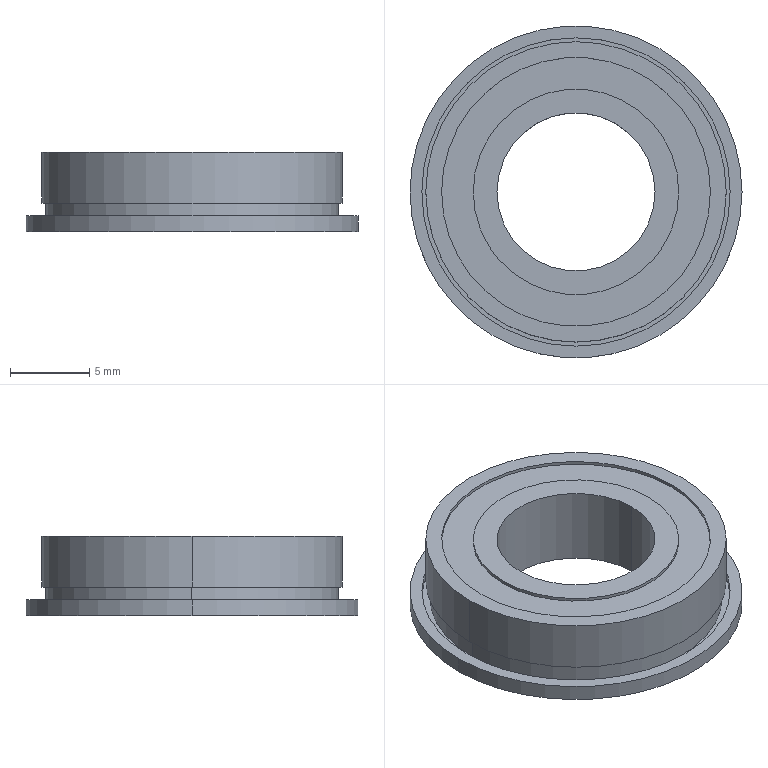Part | STEP file | 202-01-0017 | 1 solid | 27 faces | box 21 x 21 x 5 mm | volume 1023 mm3 | cylinder 18 | plane 9 | commonest cylinder face diameters 13 x4 17 x4 10 x2 18.5 x2 19 x2 19.5 x2